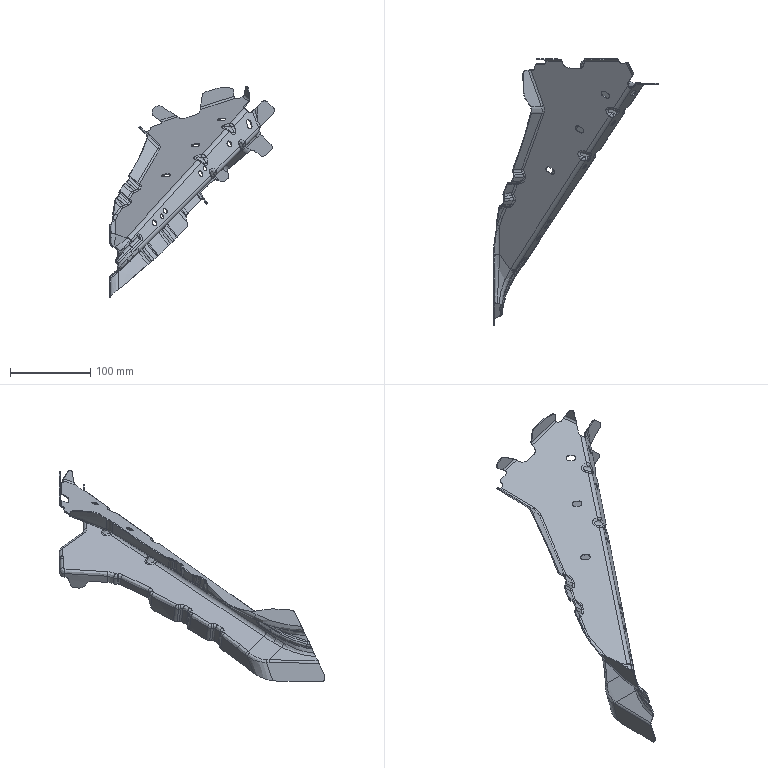Part | 1 solid | 626 faces | box 204.978 x 330.713 x 263.182 mm | volume 77320 mm3 | spline 499 | cylinder 82 | plane 37 | sphere 4 | torus 4 | commonest cylinder face diameters 10 x13 6 x12 8 x8 8.4 x8 12 x7 9.6 x6